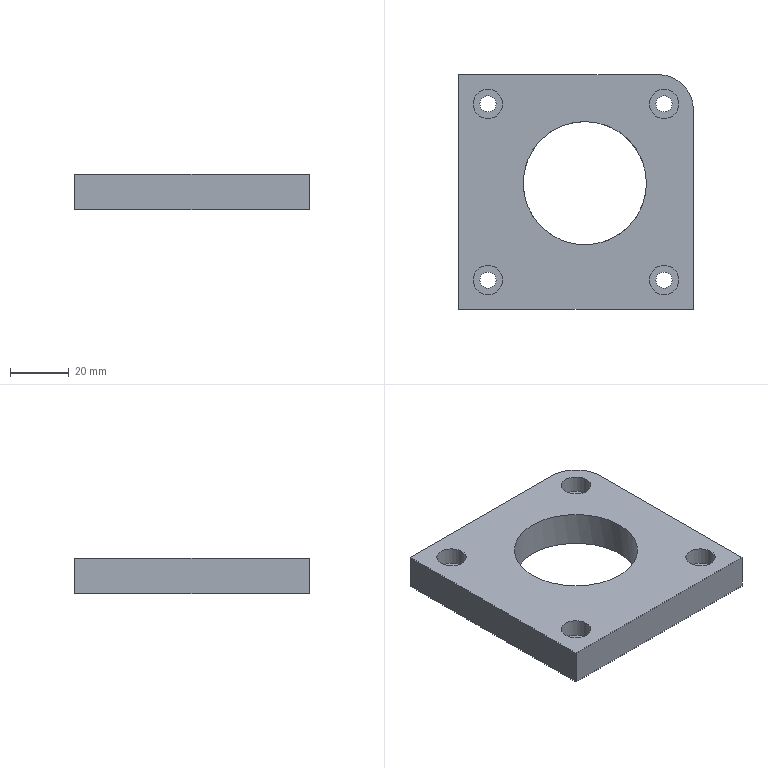Part | STEP file | solid 82 | 1 solid | 20 faces | box 80 x 80 x 12 mm | volume 57349 mm3 | plane 10 | cylinder 10 | commonest cylinder face diameters 5.5 x4 10 x4 24 x1 42 x1